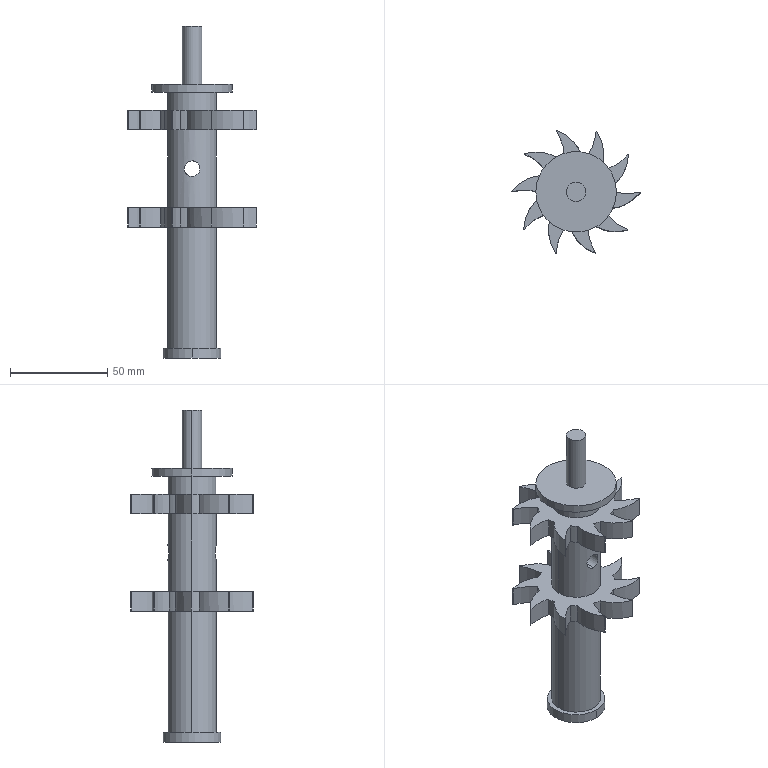Part | SolidWorks | features ICE 7, Cut 1, Extrusion 1, MirrorSolid 1 | 1 solid | 118 faces | box 65.926 x 62.827 x 170.5 mm | volume 102049 mm3 | cylinder 68 | spline 40 | plane 10 | commonest cylinder face diameters 0.4 x32 40 x20 25 x8 8 x2 10 x2 29.709 x2